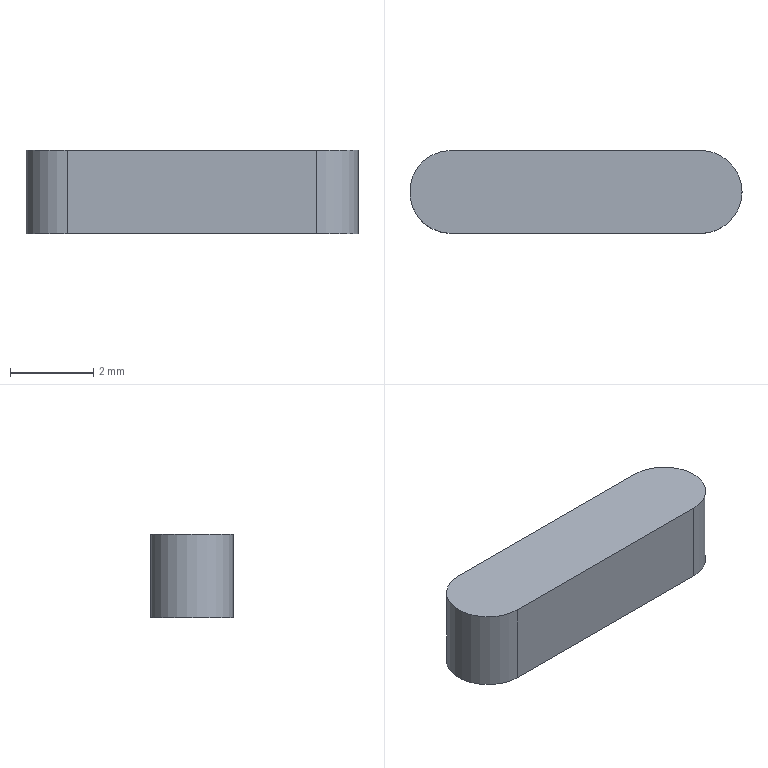Part | STEP file | BLC01-B2-L8 | 1 solid | 7 faces | box 8 x 2 x 2 mm | volume 30.283 mm3 | plane 4 | cylinder 3 | commonest cylinder face diameters 2 x3
STEP:
#1=CARTESIAN_POINT('',(0.,0.,0.));
#2=DIRECTION('',(0.,0.,1.));
#3=DIRECTION('',(1.,0.,0.));
#4=AXIS2_PLACEMENT_3D('',#1,#2,#3);
#5=CARTESIAN_POINT('',(3.,-1.,0.));
#6=VERTEX_POINT('',#5);
#7=CARTESIAN_POINT('',(4.,0.,0.));
#8=VERTEX_POINT('',#7);
#9=CARTESIAN_POINT('',(3.,0.,0.));
#10=DIRECTION('',(0.,0.,1.));
#11=DIRECTION('',(1.,0.,0.));
#12=AXIS2_PLACEMENT_3D('',#9,#10,#11);
#13=CIRCLE('',#12,1.);
#14=CARTESIAN_POINT('',(3.,0.,2.));
#15=DIRECTION('',(0.,0.,1.));
#16=DIRECTION('',(1.,0.,0.));
#17=AXIS2_PLACEMENT_3D('',#14,#15,#16);
#18=CYLINDRICAL_SURFACE('',#17,1.);
#19=CARTESIAN_POINT('',(0.,-2.));
#20=DIRECTION('',(1.,0.));
#21=VECTOR('',#20,1.);
#22=LINE('',#19,#21);
#23=(GEOMETRIC_REPRESENTATION_CONTEXT(2)PARAMETRIC_REPRESENTATION_CONTEXT()REPRESENTATION_CONTEXT('',''));
#24=DEFINITIONAL_REPRESENTATION('',(#22),#23);
#25=PCURVE('',#18,#24);
#26=CARTESIAN_POINT('',(-3.,0.,0.));
#27=DIRECTION('',(0.,0.,1.));
#28=DIRECTION('',(1.,0.,0.));
#29=AXIS2_PLACEMENT_3D('',#26,#27,#28);
#30=PLANE('',#29);
#31=CARTESIAN_POINT('',(6.,0.));
#32=DIRECTION('',(1.,0.));
#33=AXIS2_PLACEMENT_2D('',#31,#32);
#34=CIRCLE('',#33,1.);
#35=(GEOMETRIC_REPRESENTATION_CONTEXT(2)PARAMETRIC_REPRESENTATION_CONTEXT()REPRESENTATION_CONTEXT('',''));
#36=DEFINITIONAL_REPRESENTATION('',(#34),#35);
#37=PCURVE('',#30,#36);
#38=SURFACE_CURVE('',#13,(#25,#37),.PCURVE_S1.);
#39=EDGE_CURVE('',#6,#8,#38,.T.);
#40=ORIENTED_EDGE('',*,*,#39,.T.);
#41=CARTESIAN_POINT('',(4.,0.,2.));
#42=VERTEX_POINT('',#41);
#43=CARTESIAN_POINT('',(4.,0.,2.));
#44=DIRECTION('',(0.,0.,1.));
#45=VECTOR('',#44,1.);
#46=LINE('',#43,#45);
#47=CARTESIAN_POINT('',(6.283,0.));
#48=DIRECTION('',(0.,1.));
#49=VECTOR('',#48,1.);
#50=LINE('',#47,#49);
#51=(GEOMETRIC_REPRESENTATION_CONTEXT(2)PARAMETRIC_REPRESENTATION_CONTEXT()REPRESENTATION_CONTEXT('',''));
#52=DEFINITIONAL_REPRESENTATION('',(#50),#51);
#53=PCURVE('',#18,#52);
#54=CARTESIAN_POINT('',(3.,0.,2.));
#55=DIRECTION('',(0.,0.,1.));
#56=DIRECTION('',(1.,0.,0.));
#57=AXIS2_PLACEMENT_3D('',#54,#55,#56);
#58=CYLINDRICAL_SURFACE('',#57,1.);
#59=CARTESIAN_POINT('',(0.,0.));
#60=DIRECTION('',(0.,1.));
#61=VECTOR('',#60,1.);
#62=LINE('',#59,#61);
#63=(GEOMETRIC_REPRESENTATION_CONTEXT(2)PARAMETRIC_REPRESENTATION_CONTEXT()REPRESENTATION_CONTEXT('',''));
#64=DEFINITIONAL_REPRESENTATION('',(#62),#63);
#65=PCURVE('',#58,#64);
#66=SURFACE_CURVE('',#46,(#53,#65),.PCURVE_S1.);
#67=EDGE_CURVE('',#8,#42,#66,.T.);
#68=ORIENTED_EDGE('',*,*,#67,.T.);
#69=CARTESIAN_POINT('',(3.,-1.,2.));
#70=VERTEX_POINT('',#69);
#71=CARTESIAN_POINT('',(3.,0.,2.));
#72=DIRECTION('',(0.,0.,-1.));
#73=DIRECTION('',(1.,0.,0.));
#74=AXIS2_PLACEMENT_3D('',#71,#72,#73);
#75=CIRCLE('',#74,1.);
#76=CARTESIAN_POINT('',(6.283,0.));
#77=DIRECTION('',(-1.,0.));
#78=VECTOR('',#77,1.);
#79=LINE('',#76,#78);
#80=(GEOMETRIC_REPRESENTATION_CONTEXT(2)PARAMETRIC_REPRESENTATION_CONTEXT()REPRESENTATION_CONTEXT('',''));
#81=DEFINITIONAL_REPRESENTATION('',(#79),#80);
#82=PCURVE('',#18,#81);
#83=CARTESIAN_POINT('',(-3.,0.,2.));
#84=DIRECTION('',(0.,0.,1.));
#85=DIRECTION('',(1.,0.,0.));
#86=AXIS2_PLACEMENT_3D('',#83,#84,#85);
#87=PLANE('',#86);
#88=CARTESIAN_POINT('',(7.,0.));
#89=CARTESIAN_POINT('',(7.,-1.732));
#90=CARTESIAN_POINT('',(5.5,-0.866));
#91=CARTESIAN_POINT('',(4.,0.));
#92=CARTESIAN_POINT('',(5.5,0.866));
#93=CARTESIAN_POINT('',(7.,1.732));
#94=CARTESIAN_POINT('',(7.,0.));
#95=(BOUNDED_CURVE()B_SPLINE_CURVE(2,(#88,#89,#90,#91,#92,#93,#94),.UNSPECIFIED.,.T.,.F.)B_SPLINE_CURVE_WITH_KNOTS((1,2,2,2,2,1),(-2.094,0.,2.094,4.189,6.283,8.378),.UNSPECIFIED.)CURVE()GEOMETRIC_REPRESENTATION_ITEM()RATIONAL_B_SPLINE_CURVE((1.,0.5,1.,0.5,1.,0.5,1.))REPRESENTATION_ITEM(''));
#96=(GEOMETRIC_REPRESENTATION_CONTEXT(2)PARAMETRIC_REPRESENTATION_CONTEXT()REPRESENTATION_CONTEXT('',''));
#97=DEFINITIONAL_REPRESENTATION('',(#95),#96);
#98=PCURVE('',#87,#97);
#99=SURFACE_CURVE('',#75,(#82,#98),.PCURVE_S1.);
#100=EDGE_CURVE('',#42,#70,#99,.T.);
#101=ORIENTED_EDGE('',*,*,#100,.T.);
#102=CARTESIAN_POINT('',(3.,-1.,2.));
#103=DIRECTION('',(0.,0.,-1.));
#104=VECTOR('',#103,1.);
#105=LINE('',#102,#104);
#106=CARTESIAN_POINT('',(4.712,0.));
#107=DIRECTION('',(0.,-1.));
#108=VECTOR('',#107,1.);
#109=LINE('',#106,#108);
#110=(GEOMETRIC_REPRESENTATION_CONTEXT(2)PARAMETRIC_REPRESENTATION_CONTEXT()REPRESENTATION_CONTEXT('',''));
#111=DEFINITIONAL_REPRESENTATION('',(#109),#110);
#112=PCURVE('',#18,#111);
#113=CARTESIAN_POINT('',(-3.,-1.,2.));
#114=DIRECTION('',(0.,1.,0.));
#115=DIRECTION('',(0.,0.,1.));
#116=AXIS2_PLACEMENT_3D('',#113,#114,#115);
#117=PLANE('',#116);
#118=CARTESIAN_POINT('',(0.,6.));
#119=DIRECTION('',(-1.,0.));
#120=VECTOR('',#119,1.);
#121=LINE('',#118,#120);
#122=(GEOMETRIC_REPRESENTATION_CONTEXT(2)PARAMETRIC_REPRESENTATION_CONTEXT()REPRESENTATION_CONTEXT('',''));
#123=DEFINITIONAL_REPRESENTATION('',(#121),#122);
#124=PCURVE('',#117,#123);
#125=SURFACE_CURVE('',#105,(#112,#124),.PCURVE_S1.);
#126=EDGE_CURVE('',#70,#6,#125,.T.);
#127=ORIENTED_EDGE('',*,*,#126,.T.);
#128=EDGE_LOOP('',(#40,#68,#101,#127));
#129=FACE_BOUND('',#128,.T.);
#130=ADVANCED_FACE('',(#129),#18,.T.);
#131=ORIENTED_EDGE('',*,*,#39,.F.);
#132=CARTESIAN_POINT('',(-3.,-1.,0.));
#133=VERTEX_POINT('',#132);
#134=CARTESIAN_POINT('',(-3.,-1.,0.));
#135=DIRECTION('',(1.,0.,0.));
#136=VECTOR('',#135,1.);
#137=LINE('',#134,#136);
#138=CARTESIAN_POINT('',(0.,-1.));
#139=DIRECTION('',(1.,0.));
#140=VECTOR('',#139,1.);
#141=LINE('',#138,#140);
#142=(GEOMETRIC_REPRESENTATION_CONTEXT(2)PARAMETRIC_REPRESENTATION_CONTEXT()REPRESENTATION_CONTEXT('',''));
#143=DEFINITIONAL_REPRESENTATION('',(#141),#142);
#144=PCURVE('',#30,#143);
#145=CARTESIAN_POINT('',(-2.,0.));
#146=DIRECTION('',(0.,1.));
#147=VECTOR('',#146,1.);
#148=LINE('',#145,#147);
#149=(GEOMETRIC_REPRESENTATION_CONTEXT(2)PARAMETRIC_REPRESENTATION_CONTEXT()REPRESENTATION_CONTEXT('',''));
#150=DEFINITIONAL_REPRESENTATION('',(#148),#149);
#151=PCURVE('',#117,#150);
#152=SURFACE_CURVE('',#137,(#144,#151),.PCURVE_S1.);
#153=EDGE_CURVE('',#133,#6,#152,.T.);
#154=ORIENTED_EDGE('',*,*,#153,.F.);
#155=CARTESIAN_POINT('',(-3.,1.,0.));
#156=VERTEX_POINT('',#155);
#157=CARTESIAN_POINT('',(-3.,0.,0.));
#158=DIRECTION('',(0.,0.,1.));
#159=DIRECTION('',(1.,0.,0.));
#160=AXIS2_PLACEMENT_3D('',#157,#158,#159);
#161=CIRCLE('',#160,1.);
#162=CARTESIAN_POINT('',(0.,0.));
#163=DIRECTION('',(1.,0.));
#164=AXIS2_PLACEMENT_2D('',#162,#163);
#165=CIRCLE('',#164,1.);
#166=(GEOMETRIC_REPRESENTATION_CONTEXT(2)PARAMETRIC_REPRESENTATION_CONTEXT()REPRESENTATION_CONTEXT('',''));
#167=DEFINITIONAL_REPRESENTATION('',(#165),#166);
#168=PCURVE('',#30,#167);
#169=CARTESIAN_POINT('',(-3.,0.,2.));
#170=DIRECTION('',(0.,0.,1.));
#171=DIRECTION('',(1.,0.,0.));
#172=AXIS2_PLACEMENT_3D('',#169,#170,#171);
#173=CYLINDRICAL_SURFACE('',#172,1.);
#174=CARTESIAN_POINT('',(0.,-2.));
#175=DIRECTION('',(1.,0.));
#176=VECTOR('',#175,1.);
#177=LINE('',#174,#176);
#178=(GEOMETRIC_REPRESENTATION_CONTEXT(2)PARAMETRIC_REPRESENTATION_CONTEXT()REPRESENTATION_CONTEXT('',''));
#179=DEFINITIONAL_REPRESENTATION('',(#177),#178);
#180=PCURVE('',#173,#179);
#181=SURFACE_CURVE('',#161,(#168,#180),.PCURVE_S1.);
#182=EDGE_CURVE('',#156,#133,#181,.T.);
#183=ORIENTED_EDGE('',*,*,#182,.F.);
#184=CARTESIAN_POINT('',(3.,1.,0.));
#185=VERTEX_POINT('',#184);
#186=CARTESIAN_POINT('',(-3.,1.,0.));
#187=DIRECTION('',(-1.,0.,0.));
#188=VECTOR('',#187,1.);
#189=LINE('',#186,#188);
#190=CARTESIAN_POINT('',(0.,1.));
#191=DIRECTION('',(-1.,0.));
#192=VECTOR('',#191,1.);
#193=LINE('',#190,#192);
#194=(GEOMETRIC_REPRESENTATION_CONTEXT(2)PARAMETRIC_REPRESENTATION_CONTEXT()REPRESENTATION_CONTEXT('',''));
#195=DEFINITIONAL_REPRESENTATION('',(#193),#194);
#196=PCURVE('',#30,#195);
#197=CARTESIAN_POINT('',(3.,1.,2.));
#198=DIRECTION('',(0.,-1.,0.));
#199=DIRECTION('',(0.,0.,-1.));
#200=AXIS2_PLACEMENT_3D('',#197,#198,#199);
#201=PLANE('',#200);
#202=CARTESIAN_POINT('',(2.,-6.));
#203=DIRECTION('',(0.,-1.));
#204=VECTOR('',#203,1.);
#205=LINE('',#202,#204);
#206=(GEOMETRIC_REPRESENTATION_CONTEXT(2)PARAMETRIC_REPRESENTATION_CONTEXT()REPRESENTATION_CONTEXT('',''));
#207=DEFINITIONAL_REPRESENTATION('',(#205),#206);
#208=PCURVE('',#201,#207);
#209=SURFACE_CURVE('',#189,(#196,#208),.PCURVE_S1.);
#210=EDGE_CURVE('',#185,#156,#209,.T.);
#211=ORIENTED_EDGE('',*,*,#210,.F.);
#212=CARTESIAN_POINT('',(3.,0.,0.));
#213=DIRECTION('',(0.,0.,1.));
#214=DIRECTION('',(1.,0.,0.));
#215=AXIS2_PLACEMENT_3D('',#212,#213,#214);
#216=CIRCLE('',#215,1.);
#217=CARTESIAN_POINT('',(6.,0.));
#218=DIRECTION('',(1.,0.));
#219=AXIS2_PLACEMENT_2D('',#217,#218);
#220=CIRCLE('',#219,1.);
#221=(GEOMETRIC_REPRESENTATION_CONTEXT(2)PARAMETRIC_REPRESENTATION_CONTEXT()REPRESENTATION_CONTEXT('',''));
#222=DEFINITIONAL_REPRESENTATION('',(#220),#221);
#223=PCURVE('',#30,#222);
#224=CARTESIAN_POINT('',(0.,-2.));
#225=DIRECTION('',(1.,0.));
#226=VECTOR('',#225,1.);
#227=LINE('',#224,#226);
#228=(GEOMETRIC_REPRESENTATION_CONTEXT(2)PARAMETRIC_REPRESENTATION_CONTEXT()REPRESENTATION_CONTEXT('',''));
#229=DEFINITIONAL_REPRESENTATION('',(#227),#228);
#230=PCURVE('',#58,#229);
#231=SURFACE_CURVE('',#216,(#223,#230),.PCURVE_S1.);
#232=EDGE_CURVE('',#8,#185,#231,.T.);
#233=ORIENTED_EDGE('',*,*,#232,.F.);
#234=EDGE_LOOP('',(#131,#154,#183,#211,#233));
#235=FACE_BOUND('',#234,.T.);
#236=ADVANCED_FACE('',(#235),#30,.F.);
#237=CARTESIAN_POINT('',(-3.,1.,2.));
#238=VERTEX_POINT('',#237);
#239=CARTESIAN_POINT('',(-3.,1.,2.));
#240=DIRECTION('',(0.,0.,-1.));
#241=VECTOR('',#240,1.);
#242=LINE('',#239,#241);
#243=CARTESIAN_POINT('',(0.,-6.));
#244=DIRECTION('',(1.,0.));
#245=VECTOR('',#244,1.);
#246=LINE('',#243,#245);
#247=(GEOMETRIC_REPRESENTATION_CONTEXT(2)PARAMETRIC_REPRESENTATION_CONTEXT()REPRESENTATION_CONTEXT('',''));
#248=DEFINITIONAL_REPRESENTATION('',(#246),#247);
#249=PCURVE('',#201,#248);
#250=CARTESIAN_POINT('',(1.571,0.));
#251=DIRECTION('',(0.,-1.));
#252=VECTOR('',#251,1.);
#253=LINE('',#250,#252);
#254=(GEOMETRIC_REPRESENTATION_CONTEXT(2)PARAMETRIC_REPRESENTATION_CONTEXT()REPRESENTATION_CONTEXT('',''));
#255=DEFINITIONAL_REPRESENTATION('',(#253),#254);
#256=PCURVE('',#173,#255);
#257=SURFACE_CURVE('',#242,(#249,#256),.PCURVE_S1.);
#258=EDGE_CURVE('',#238,#156,#257,.T.);
#259=ORIENTED_EDGE('',*,*,#258,.F.);
#260=CARTESIAN_POINT('',(3.,1.,2.));
#261=VERTEX_POINT('',#260);
#262=CARTESIAN_POINT('',(3.,1.,2.));
#263=DIRECTION('',(-1.,0.,0.));
#264=VECTOR('',#263,1.);
#265=LINE('',#262,#264);
#266=CARTESIAN_POINT('',(0.,0.));
#267=DIRECTION('',(0.,-1.));
#268=VECTOR('',#267,1.);
#269=LINE('',#266,#268);
#270=(GEOMETRIC_REPRESENTATION_CONTEXT(2)PARAMETRIC_REPRESENTATION_CONTEXT()REPRESENTATION_CONTEXT('',''));
#271=DEFINITIONAL_REPRESENTATION('',(#269),#270);
#272=PCURVE('',#201,#271);
#273=CARTESIAN_POINT('',(6.,1.));
#274=DIRECTION('',(-1.,0.));
#275=VECTOR('',#274,1.);
#276=LINE('',#273,#275);
#277=(GEOMETRIC_REPRESENTATION_CONTEXT(2)PARAMETRIC_REPRESENTATION_CONTEXT()REPRESENTATION_CONTEXT('',''));
#278=DEFINITIONAL_REPRESENTATION('',(#276),#277);
#279=PCURVE('',#87,#278);
#280=SURFACE_CURVE('',#265,(#272,#279),.PCURVE_S1.);
#281=EDGE_CURVE('',#261,#238,#280,.T.);
#282=ORIENTED_EDGE('',*,*,#281,.F.);
#283=CARTESIAN_POINT('',(3.,1.,2.));
#284=DIRECTION('',(0.,0.,1.));
#285=VECTOR('',#284,1.);
#286=LINE('',#283,#285);
#287=CARTESIAN_POINT('',(0.,0.));
#288=DIRECTION('',(-1.,0.));
#289=VECTOR('',#288,1.);
#290=LINE('',#287,#289);
#291=(GEOMETRIC_REPRESENTATION_CONTEXT(2)PARAMETRIC_REPRESENTATION_CONTEXT()REPRESENTATION_CONTEXT('',''));
#292=DEFINITIONAL_REPRESENTATION('',(#290),#291);
#293=PCURVE('',#201,#292);
#294=CARTESIAN_POINT('',(1.571,0.));
#295=DIRECTION('',(0.,1.));
#296=VECTOR('',#295,1.);
#297=LINE('',#294,#296);
#298=(GEOMETRIC_REPRESENTATION_CONTEXT(2)PARAMETRIC_REPRESENTATION_CONTEXT()REPRESENTATION_CONTEXT('',''));
#299=DEFINITIONAL_REPRESENTATION('',(#297),#298);
#300=PCURVE('',#58,#299);
#301=SURFACE_CURVE('',#286,(#293,#300),.PCURVE_S1.);
#302=EDGE_CURVE('',#185,#261,#301,.T.);
#303=ORIENTED_EDGE('',*,*,#302,.F.);
#304=ORIENTED_EDGE('',*,*,#210,.T.);
#305=EDGE_LOOP('',(#259,#282,#303,#304));
#306=FACE_BOUND('',#305,.T.);
#307=ADVANCED_FACE('',(#306),#201,.F.);
#308=ORIENTED_EDGE('',*,*,#67,.F.);
#309=ORIENTED_EDGE('',*,*,#232,.T.);
#310=ORIENTED_EDGE('',*,*,#302,.T.);
#311=CARTESIAN_POINT('',(3.,0.,2.));
#312=DIRECTION('',(0.,0.,-1.));
#313=DIRECTION('',(1.,0.,0.));
#314=AXIS2_PLACEMENT_3D('',#311,#312,#313);
#315=CIRCLE('',#314,1.);
#316=CARTESIAN_POINT('',(6.283,0.));
#317=DIRECTION('',(-1.,0.));
#318=VECTOR('',#317,1.);
#319=LINE('',#316,#318);
#320=(GEOMETRIC_REPRESENTATION_CONTEXT(2)PARAMETRIC_REPRESENTATION_CONTEXT()REPRESENTATION_CONTEXT('',''));
#321=DEFINITIONAL_REPRESENTATION('',(#319),#320);
#322=PCURVE('',#58,#321);
#323=CARTESIAN_POINT('',(7.,0.));
#324=CARTESIAN_POINT('',(7.,-1.732));
#325=CARTESIAN_POINT('',(5.5,-0.866));
#326=CARTESIAN_POINT('',(4.,0.));
#327=CARTESIAN_POINT('',(5.5,0.866));
#328=CARTESIAN_POINT('',(7.,1.732));
#329=CARTESIAN_POINT('',(7.,0.));
#330=(BOUNDED_CURVE()B_SPLINE_CURVE(2,(#323,#324,#325,#326,#327,#328,#329),.UNSPECIFIED.,.T.,.F.)B_SPLINE_CURVE_WITH_KNOTS((1,2,2,2,2,1),(-2.094,0.,2.094,4.189,6.283,8.378),.UNSPECIFIED.)CURVE()GEOMETRIC_REPRESENTATION_ITEM()RATIONAL_B_SPLINE_CURVE((1.,0.5,1.,0.5,1.,0.5,1.))REPRESENTATION_ITEM(''));
#331=(GEOMETRIC_REPRESENTATION_CONTEXT(2)PARAMETRIC_REPRESENTATION_CONTEXT()REPRESENTATION_CONTEXT('',''));
#332=DEFINITIONAL_REPRESENTATION('',(#330),#331);
#333=PCURVE('',#87,#332);
#334=SURFACE_CURVE('',#315,(#322,#333),.PCURVE_S1.);
#335=EDGE_CURVE('',#261,#42,#334,.T.);
#336=ORIENTED_EDGE('',*,*,#335,.T.);
#337=EDGE_LOOP('',(#308,#309,#310,#336));
#338=FACE_BOUND('',#337,.T.);
#339=ADVANCED_FACE('',(#338),#58,.T.);
#340=ORIENTED_EDGE('',*,*,#126,.F.);
#341=CARTESIAN_POINT('',(-3.,-1.,2.));
#342=VERTEX_POINT('',#341);
#343=CARTESIAN_POINT('',(-3.,-1.,2.));
#344=DIRECTION('',(1.,0.,0.));
#345=VECTOR('',#344,1.);
#346=LINE('',#343,#345);
#347=CARTESIAN_POINT('',(0.,0.));
#348=DIRECTION('',(0.,1.));
#349=VECTOR('',#348,1.);
#350=LINE('',#347,#349);
#351=(GEOMETRIC_REPRESENTATION_CONTEXT(2)PARAMETRIC_REPRESENTATION_CONTEXT()REPRESENTATION_CONTEXT('',''));
#352=DEFINITIONAL_REPRESENTATION('',(#350),#351);
#353=PCURVE('',#117,#352);
#354=CARTESIAN_POINT('',(0.,-1.));
#355=DIRECTION('',(1.,0.));
#356=VECTOR('',#355,1.);
#357=LINE('',#354,#356);
#358=(GEOMETRIC_REPRESENTATION_CONTEXT(2)PARAMETRIC_REPRESENTATION_CONTEXT()REPRESENTATION_CONTEXT('',''));
#359=DEFINITIONAL_REPRESENTATION('',(#357),#358);
#360=PCURVE('',#87,#359);
#361=SURFACE_CURVE('',#346,(#353,#360),.PCURVE_S1.);
#362=EDGE_CURVE('',#342,#70,#361,.T.);
#363=ORIENTED_EDGE('',*,*,#362,.F.);
#364=CARTESIAN_POINT('',(-3.,-1.,2.));
#365=DIRECTION('',(0.,0.,1.));
#366=VECTOR('',#365,1.);
#367=LINE('',#364,#366);
#368=CARTESIAN_POINT('',(0.,0.));
#369=DIRECTION('',(1.,0.));
#370=VECTOR('',#369,1.);
#371=LINE('',#368,#370);
#372=(GEOMETRIC_REPRESENTATION_CONTEXT(2)PARAMETRIC_REPRESENTATION_CONTEXT()REPRESENTATION_CONTEXT('',''));
#373=DEFINITIONAL_REPRESENTATION('',(#371),#372);
#374=PCURVE('',#117,#373);
#375=CARTESIAN_POINT('',(4.712,0.));
#376=DIRECTION('',(0.,1.));
#377=VECTOR('',#376,1.);
#378=LINE('',#375,#377);
#379=(GEOMETRIC_REPRESENTATION_CONTEXT(2)PARAMETRIC_REPRESENTATION_CONTEXT()REPRESENTATION_CONTEXT('',''));
#380=DEFINITIONAL_REPRESENTATION('',(#378),#379);
#381=PCURVE('',#173,#380);
#382=SURFACE_CURVE('',#367,(#374,#381),.PCURVE_S1.);
#383=EDGE_CURVE('',#133,#342,#382,.T.);
#384=ORIENTED_EDGE('',*,*,#383,.F.);
#385=ORIENTED_EDGE('',*,*,#153,.T.);
#386=EDGE_LOOP('',(#340,#363,#384,#385));
#387=FACE_BOUND('',#386,.T.);
#388=ADVANCED_FACE('',(#387),#117,.F.);
#389=CARTESIAN_POINT('',(-3.,0.,2.));
#390=DIRECTION('',(0.,0.,-1.));
#391=DIRECTION('',(1.,0.,0.));
#392=AXIS2_PLACEMENT_3D('',#389,#390,#391);
#393=CIRCLE('',#392,1.);
#394=CARTESIAN_POINT('',(6.283,0.));
#395=DIRECTION('',(-1.,0.));
#396=VECTOR('',#395,1.);
#397=LINE('',#394,#396);
#398=(GEOMETRIC_REPRESENTATION_CONTEXT(2)PARAMETRIC_REPRESENTATION_CONTEXT()REPRESENTATION_CONTEXT('',''));
#399=DEFINITIONAL_REPRESENTATION('',(#397),#398);
#400=PCURVE('',#173,#399);
#401=CARTESIAN_POINT('',(1.,0.));
#402=CARTESIAN_POINT('',(1.,-1.732));
#403=CARTESIAN_POINT('',(-0.5,-0.866));
#404=CARTESIAN_POINT('',(-2.,0.));
#405=CARTESIAN_POINT('',(-0.5,0.866));
#406=CARTESIAN_POINT('',(1.,1.732));
#407=CARTESIAN_POINT('',(1.,0.));
#408=(BOUNDED_CURVE()B_SPLINE_CURVE(2,(#401,#402,#403,#404,#405,#406,#407),.UNSPECIFIED.,.T.,.F.)B_SPLINE_CURVE_WITH_KNOTS((1,2,2,2,2,1),(-2.094,0.,2.094,4.189,6.283,8.378),.UNSPECIFIED.)CURVE()GEOMETRIC_REPRESENTATION_ITEM()RATIONAL_B_SPLINE_CURVE((1.,0.5,1.,0.5,1.,0.5,1.))REPRESENTATION_ITEM(''));
#409=(GEOMETRIC_REPRESENTATION_CONTEXT(2)PARAMETRIC_REPRESENTATION_CONTEXT()REPRESENTATION_CONTEXT('',''));
#410=DEFINITIONAL_REPRESENTATION('',(#408),#409);
#411=PCURVE('',#87,#410);
#412=SURFACE_CURVE('',#393,(#400,#411),.PCURVE_S1.);
#413=EDGE_CURVE('',#342,#238,#412,.T.);
#414=ORIENTED_EDGE('',*,*,#413,.T.);
#415=ORIENTED_EDGE('',*,*,#258,.T.);
#416=ORIENTED_EDGE('',*,*,#182,.T.);
#417=ORIENTED_EDGE('',*,*,#383,.T.);
#418=EDGE_LOOP('',(#414,#415,#416,#417));
#419=FACE_BOUND('',#418,.T.);
#420=ADVANCED_FACE('',(#419),#173,.T.);
#421=ORIENTED_EDGE('',*,*,#362,.T.);
#422=ORIENTED_EDGE('',*,*,#100,.F.);
#423=ORIENTED_EDGE('',*,*,#335,.F.);
#424=ORIENTED_EDGE('',*,*,#281,.T.);
#425=ORIENTED_EDGE('',*,*,#413,.F.);
#426=EDGE_LOOP('',(#421,#422,#423,#424,#425));
#427=FACE_BOUND('',#426,.T.);
#428=ADVANCED_FACE('',(#427),#87,.T.);
#429=CLOSED_SHELL('',(#130,#236,#307,#339,#388,#420,#428));
#430=MANIFOLD_SOLID_BREP('',#429);
#431=(LENGTH_UNIT()NAMED_UNIT(*)SI_UNIT(.MILLI.,.METRE.));
#432=UNCERTAINTY_MEASURE_WITH_UNIT(LENGTH_MEASURE(0.0000001),#431,'','');
#433=(NAMED_UNIT(*)PLANE_ANGLE_UNIT()SI_UNIT($,.RADIAN.));
#434=(NAMED_UNIT(*)SI_UNIT($,.STERADIAN.)SOLID_ANGLE_UNIT());
#435=(GEOMETRIC_REPRESENTATION_CONTEXT(3)GLOBAL_UNCERTAINTY_ASSIGNED_CONTEXT((#432))GLOBAL_UNIT_ASSIGNED_CONTEXT((#431,#433,#434))REPRESENTATION_CONTEXT('',''));
#436=ADVANCED_BREP_SHAPE_REPRESENTATION('',(#4,#430),#435);